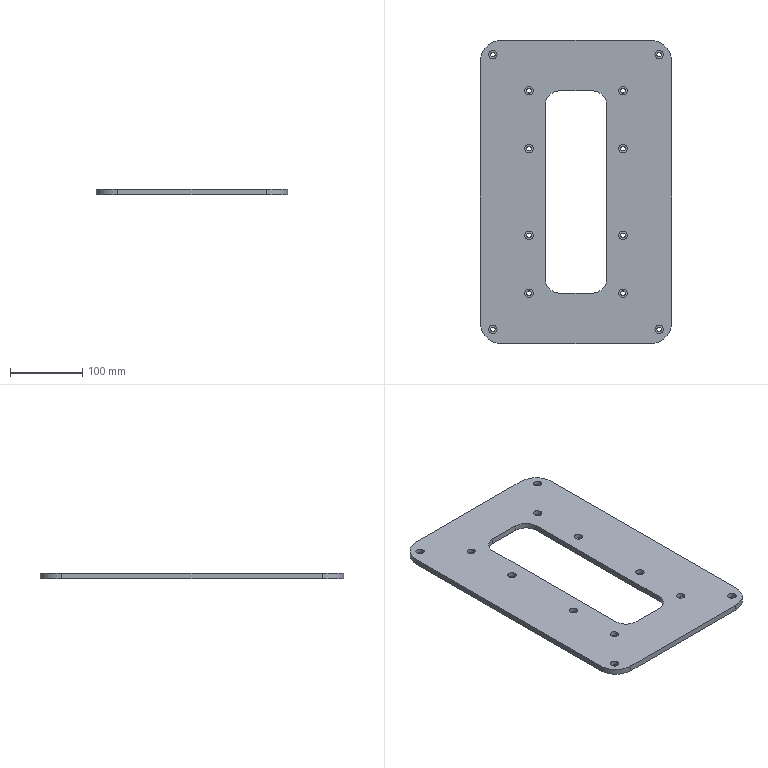Part | STEP file | SL2-MOLD_id354_xmt_txt | 1 solid | 54 faces | box 265 x 420 x 8 mm | volume 688291 mm3 | cylinder 32 | plane 22 | commonest cylinder face diameters 6.5 x12 11.5 x12 40 x4 60 x4
STEP:
#1=CARTESIAN_POINT('',(-42.5,-30.,101.));
#2=VERTEX_POINT('',#1);
#3=CARTESIAN_POINT('',(-42.5,210.,101.));
#4=VERTEX_POINT('',#3);
#5=CARTESIAN_POINT('',(-42.5,-30.,101.));
#6=DIRECTION('',(0.,1.,0.));
#7=VECTOR('',#6,1.);
#8=LINE('',#5,#7);
#9=EDGE_CURVE('',#2,#4,#8,.T.);
#10=ORIENTED_EDGE('',*,*,#9,.F.);
#11=CARTESIAN_POINT('',(-42.5,-30.,93.));
#12=VERTEX_POINT('',#11);
#13=CARTESIAN_POINT('',(-42.5,-30.,93.));
#14=DIRECTION('',(0.,0.,1.));
#15=VECTOR('',#14,1.);
#16=LINE('',#13,#15);
#17=EDGE_CURVE('',#12,#2,#16,.T.);
#18=ORIENTED_EDGE('',*,*,#17,.F.);
#19=CARTESIAN_POINT('',(-42.5,210.,93.));
#20=VERTEX_POINT('',#19);
#21=CARTESIAN_POINT('',(-42.5,-30.,93.));
#22=DIRECTION('',(0.,1.,0.));
#23=VECTOR('',#22,1.);
#24=LINE('',#21,#23);
#25=EDGE_CURVE('',#12,#20,#24,.T.);
#26=ORIENTED_EDGE('',*,*,#25,.T.);
#27=CARTESIAN_POINT('',(-42.5,210.,93.));
#28=DIRECTION('',(0.,0.,1.));
#29=VECTOR('',#28,1.);
#30=LINE('',#27,#29);
#31=EDGE_CURVE('',#20,#4,#30,.T.);
#32=ORIENTED_EDGE('',*,*,#31,.T.);
#33=EDGE_LOOP('',(#10,#18,#26,#32));
#34=FACE_OUTER_BOUND('',#33,.T.);
#35=CARTESIAN_POINT('',(-42.5,-30.,93.));
#36=DIRECTION('',(1.,0.,0.));
#37=DIRECTION('',(0.,1.,0.));
#38=AXIS2_PLACEMENT_3D('',#35,#36,#37);
#39=PLANE('',#38);
#40=ADVANCED_FACE('',(#34),#39,.T.);
#41=CARTESIAN_POINT('',(-22.5,-50.,101.));
#42=VERTEX_POINT('',#41);
#43=CARTESIAN_POINT('',(-22.5,-30.,101.));
#44=DIRECTION('',(0.,0.,-1.));
#45=DIRECTION('',(1.,0.,0.));
#46=AXIS2_PLACEMENT_3D('',#43,#44,#45);
#47=CIRCLE('',#46,20.);
#48=EDGE_CURVE('',#42,#2,#47,.T.);
#49=ORIENTED_EDGE('',*,*,#48,.F.);
#50=CARTESIAN_POINT('',(-22.5,-50.,93.));
#51=VERTEX_POINT('',#50);
#52=CARTESIAN_POINT('',(-22.5,-50.,93.));
#53=DIRECTION('',(0.,0.,1.));
#54=VECTOR('',#53,1.);
#55=LINE('',#52,#54);
#56=EDGE_CURVE('',#51,#42,#55,.T.);
#57=ORIENTED_EDGE('',*,*,#56,.F.);
#58=CARTESIAN_POINT('',(-22.5,-30.,93.));
#59=DIRECTION('',(0.,0.,-1.));
#60=DIRECTION('',(1.,0.,0.));
#61=AXIS2_PLACEMENT_3D('',#58,#59,#60);
#62=CIRCLE('',#61,20.);
#63=EDGE_CURVE('',#51,#12,#62,.T.);
#64=ORIENTED_EDGE('',*,*,#63,.T.);
#65=ORIENTED_EDGE('',*,*,#17,.T.);
#66=EDGE_LOOP('',(#49,#57,#64,#65));
#67=FACE_OUTER_BOUND('',#66,.T.);
#68=CARTESIAN_POINT('',(-22.5,-30.,93.));
#69=DIRECTION('',(0.,0.,1.));
#70=DIRECTION('',(1.,0.,0.));
#71=AXIS2_PLACEMENT_3D('',#68,#69,#70);
#72=CYLINDRICAL_SURFACE('',#71,20.);
#73=ADVANCED_FACE('',(#67),#72,.F.);
#74=CARTESIAN_POINT('',(22.5,-50.,101.));
#75=VERTEX_POINT('',#74);
#76=CARTESIAN_POINT('',(22.5,-50.,101.));
#77=DIRECTION('',(-1.,0.,0.));
#78=VECTOR('',#77,1.);
#79=LINE('',#76,#78);
#80=EDGE_CURVE('',#75,#42,#79,.T.);
#81=ORIENTED_EDGE('',*,*,#80,.F.);
#82=CARTESIAN_POINT('',(22.5,-50.,93.));
#83=VERTEX_POINT('',#82);
#84=CARTESIAN_POINT('',(22.5,-50.,93.));
#85=DIRECTION('',(0.,0.,1.));
#86=VECTOR('',#85,1.);
#87=LINE('',#84,#86);
#88=EDGE_CURVE('',#83,#75,#87,.T.);
#89=ORIENTED_EDGE('',*,*,#88,.F.);
#90=CARTESIAN_POINT('',(22.5,-50.,93.));
#91=DIRECTION('',(-1.,0.,0.));
#92=VECTOR('',#91,1.);
#93=LINE('',#90,#92);
#94=EDGE_CURVE('',#83,#51,#93,.T.);
#95=ORIENTED_EDGE('',*,*,#94,.T.);
#96=ORIENTED_EDGE('',*,*,#56,.T.);
#97=EDGE_LOOP('',(#81,#89,#95,#96));
#98=FACE_OUTER_BOUND('',#97,.T.);
#99=CARTESIAN_POINT('',(22.5,-50.,93.));
#100=DIRECTION('',(0.,1.,0.));
#101=DIRECTION('',(0.,0.,1.));
#102=AXIS2_PLACEMENT_3D('',#99,#100,#101);
#103=PLANE('',#102);
#104=ADVANCED_FACE('',(#98),#103,.T.);
#105=CARTESIAN_POINT('',(42.5,-30.,101.));
#106=VERTEX_POINT('',#105);
#107=CARTESIAN_POINT('',(22.5,-30.,101.));
#108=DIRECTION('',(0.,0.,-1.));
#109=DIRECTION('',(1.,0.,0.));
#110=AXIS2_PLACEMENT_3D('',#107,#108,#109);
#111=CIRCLE('',#110,20.);
#112=EDGE_CURVE('',#106,#75,#111,.T.);
#113=ORIENTED_EDGE('',*,*,#112,.F.);
#114=CARTESIAN_POINT('',(42.5,-30.,93.));
#115=VERTEX_POINT('',#114);
#116=CARTESIAN_POINT('',(42.5,-30.,93.));
#117=DIRECTION('',(0.,0.,1.));
#118=VECTOR('',#117,1.);
#119=LINE('',#116,#118);
#120=EDGE_CURVE('',#115,#106,#119,.T.);
#121=ORIENTED_EDGE('',*,*,#120,.F.);
#122=CARTESIAN_POINT('',(22.5,-30.,93.));
#123=DIRECTION('',(0.,0.,-1.));
#124=DIRECTION('',(1.,0.,0.));
#125=AXIS2_PLACEMENT_3D('',#122,#123,#124);
#126=CIRCLE('',#125,20.);
#127=EDGE_CURVE('',#115,#83,#126,.T.);
#128=ORIENTED_EDGE('',*,*,#127,.T.);
#129=ORIENTED_EDGE('',*,*,#88,.T.);
#130=EDGE_LOOP('',(#113,#121,#128,#129));
#131=FACE_OUTER_BOUND('',#130,.T.);
#132=CARTESIAN_POINT('',(22.5,-30.,93.));
#133=DIRECTION('',(0.,0.,1.));
#134=DIRECTION('',(1.,0.,0.));
#135=AXIS2_PLACEMENT_3D('',#132,#133,#134);
#136=CYLINDRICAL_SURFACE('',#135,20.);
#137=ADVANCED_FACE('',(#131),#136,.F.);
#138=CARTESIAN_POINT('',(42.5,210.,101.));
#139=VERTEX_POINT('',#138);
#140=CARTESIAN_POINT('',(42.5,210.,101.));
#141=DIRECTION('',(0.,-1.,0.));
#142=VECTOR('',#141,1.);
#143=LINE('',#140,#142);
#144=EDGE_CURVE('',#139,#106,#143,.T.);
#145=ORIENTED_EDGE('',*,*,#144,.F.);
#146=CARTESIAN_POINT('',(42.5,210.,93.));
#147=VERTEX_POINT('',#146);
#148=CARTESIAN_POINT('',(42.5,210.,93.));
#149=DIRECTION('',(0.,0.,1.));
#150=VECTOR('',#149,1.);
#151=LINE('',#148,#150);
#152=EDGE_CURVE('',#147,#139,#151,.T.);
#153=ORIENTED_EDGE('',*,*,#152,.F.);
#154=CARTESIAN_POINT('',(42.5,210.,93.));
#155=DIRECTION('',(0.,-1.,0.));
#156=VECTOR('',#155,1.);
#157=LINE('',#154,#156);
#158=EDGE_CURVE('',#147,#115,#157,.T.);
#159=ORIENTED_EDGE('',*,*,#158,.T.);
#160=ORIENTED_EDGE('',*,*,#120,.T.);
#161=EDGE_LOOP('',(#145,#153,#159,#160));
#162=FACE_OUTER_BOUND('',#161,.T.);
#163=CARTESIAN_POINT('',(42.5,210.,93.));
#164=DIRECTION('',(-1.,0.,0.));
#165=DIRECTION('',(0.,-1.,0.));
#166=AXIS2_PLACEMENT_3D('',#163,#164,#165);
#167=PLANE('',#166);
#168=ADVANCED_FACE('',(#162),#167,.T.);
#169=CARTESIAN_POINT('',(22.5,230.,101.));
#170=VERTEX_POINT('',#169);
#171=CARTESIAN_POINT('',(22.5,210.,101.));
#172=DIRECTION('',(0.,0.,-1.));
#173=DIRECTION('',(1.,0.,0.));
#174=AXIS2_PLACEMENT_3D('',#171,#172,#173);
#175=CIRCLE('',#174,20.);
#176=EDGE_CURVE('',#170,#139,#175,.T.);
#177=ORIENTED_EDGE('',*,*,#176,.F.);
#178=CARTESIAN_POINT('',(22.5,230.,93.));
#179=VERTEX_POINT('',#178);
#180=CARTESIAN_POINT('',(22.5,230.,93.));
#181=DIRECTION('',(0.,0.,1.));
#182=VECTOR('',#181,1.);
#183=LINE('',#180,#182);
#184=EDGE_CURVE('',#179,#170,#183,.T.);
#185=ORIENTED_EDGE('',*,*,#184,.F.);
#186=CARTESIAN_POINT('',(22.5,210.,93.));
#187=DIRECTION('',(0.,0.,-1.));
#188=DIRECTION('',(1.,0.,0.));
#189=AXIS2_PLACEMENT_3D('',#186,#187,#188);
#190=CIRCLE('',#189,20.);
#191=EDGE_CURVE('',#179,#147,#190,.T.);
#192=ORIENTED_EDGE('',*,*,#191,.T.);
#193=ORIENTED_EDGE('',*,*,#152,.T.);
#194=EDGE_LOOP('',(#177,#185,#192,#193));
#195=FACE_OUTER_BOUND('',#194,.T.);
#196=CARTESIAN_POINT('',(22.5,210.,93.));
#197=DIRECTION('',(0.,0.,1.));
#198=DIRECTION('',(1.,0.,0.));
#199=AXIS2_PLACEMENT_3D('',#196,#197,#198);
#200=CYLINDRICAL_SURFACE('',#199,20.);
#201=ADVANCED_FACE('',(#195),#200,.F.);
#202=CARTESIAN_POINT('',(-22.5,230.,101.));
#203=VERTEX_POINT('',#202);
#204=CARTESIAN_POINT('',(-22.5,230.,101.));
#205=DIRECTION('',(1.,0.,0.));
#206=VECTOR('',#205,1.);
#207=LINE('',#204,#206);
#208=EDGE_CURVE('',#203,#170,#207,.T.);
#209=ORIENTED_EDGE('',*,*,#208,.F.);
#210=CARTESIAN_POINT('',(-22.5,230.,93.));
#211=VERTEX_POINT('',#210);
#212=CARTESIAN_POINT('',(-22.5,230.,93.));
#213=DIRECTION('',(0.,0.,1.));
#214=VECTOR('',#213,1.);
#215=LINE('',#212,#214);
#216=EDGE_CURVE('',#211,#203,#215,.T.);
#217=ORIENTED_EDGE('',*,*,#216,.F.);
#218=CARTESIAN_POINT('',(-22.5,230.,93.));
#219=DIRECTION('',(1.,0.,0.));
#220=VECTOR('',#219,1.);
#221=LINE('',#218,#220);
#222=EDGE_CURVE('',#211,#179,#221,.T.);
#223=ORIENTED_EDGE('',*,*,#222,.T.);
#224=ORIENTED_EDGE('',*,*,#184,.T.);
#225=EDGE_LOOP('',(#209,#217,#223,#224));
#226=FACE_OUTER_BOUND('',#225,.T.);
#227=CARTESIAN_POINT('',(-22.5,230.,93.));
#228=DIRECTION('',(0.,-1.,0.));
#229=DIRECTION('',(0.,0.,-1.));
#230=AXIS2_PLACEMENT_3D('',#227,#228,#229);
#231=PLANE('',#230);
#232=ADVANCED_FACE('',(#226),#231,.T.);
#233=CARTESIAN_POINT('',(-102.5,300.,101.));
#234=VERTEX_POINT('',#233);
#235=CARTESIAN_POINT('',(102.5,300.,101.));
#236=VERTEX_POINT('',#235);
#237=CARTESIAN_POINT('',(-102.5,300.,101.));
#238=DIRECTION('',(1.,0.,0.));
#239=VECTOR('',#238,1.);
#240=LINE('',#237,#239);
#241=EDGE_CURVE('',#234,#236,#240,.T.);
#242=ORIENTED_EDGE('',*,*,#241,.T.);
#243=CARTESIAN_POINT('',(102.5,300.,93.));
#244=VERTEX_POINT('',#243);
#245=CARTESIAN_POINT('',(102.5,300.,93.));
#246=DIRECTION('',(0.,0.,1.));
#247=VECTOR('',#246,1.);
#248=LINE('',#245,#247);
#249=EDGE_CURVE('',#244,#236,#248,.T.);
#250=ORIENTED_EDGE('',*,*,#249,.F.);
#251=CARTESIAN_POINT('',(-102.5,300.,93.));
#252=VERTEX_POINT('',#251);
#253=CARTESIAN_POINT('',(-102.5,300.,93.));
#254=DIRECTION('',(1.,0.,0.));
#255=VECTOR('',#254,1.);
#256=LINE('',#253,#255);
#257=EDGE_CURVE('',#252,#244,#256,.T.);
#258=ORIENTED_EDGE('',*,*,#257,.F.);
#259=CARTESIAN_POINT('',(-102.5,300.,93.));
#260=DIRECTION('',(0.,0.,1.));
#261=VECTOR('',#260,1.);
#262=LINE('',#259,#261);
#263=EDGE_CURVE('',#252,#234,#262,.T.);
#264=ORIENTED_EDGE('',*,*,#263,.T.);
#265=EDGE_LOOP('',(#242,#250,#258,#264));
#266=FACE_OUTER_BOUND('',#265,.T.);
#267=CARTESIAN_POINT('',(-102.5,300.,93.));
#268=DIRECTION('',(0.,-1.,0.));
#269=DIRECTION('',(0.,0.,-1.));
#270=AXIS2_PLACEMENT_3D('',#267,#268,#269);
#271=PLANE('',#270);
#272=ADVANCED_FACE('',(#266),#271,.F.);
#273=CARTESIAN_POINT('',(132.5,270.,101.));
#274=VERTEX_POINT('',#273);
#275=CARTESIAN_POINT('',(102.5,270.,101.));
#276=DIRECTION('',(0.,0.,-1.));
#277=DIRECTION('',(1.,0.,0.));
#278=AXIS2_PLACEMENT_3D('',#275,#276,#277);
#279=CIRCLE('',#278,30.);
#280=EDGE_CURVE('',#236,#274,#279,.T.);
#281=ORIENTED_EDGE('',*,*,#280,.T.);
#282=CARTESIAN_POINT('',(132.5,270.,93.));
#283=VERTEX_POINT('',#282);
#284=CARTESIAN_POINT('',(132.5,270.,93.));
#285=DIRECTION('',(0.,0.,1.));
#286=VECTOR('',#285,1.);
#287=LINE('',#284,#286);
#288=EDGE_CURVE('',#283,#274,#287,.T.);
#289=ORIENTED_EDGE('',*,*,#288,.F.);
#290=CARTESIAN_POINT('',(102.5,270.,93.));
#291=DIRECTION('',(0.,0.,-1.));
#292=DIRECTION('',(1.,0.,0.));
#293=AXIS2_PLACEMENT_3D('',#290,#291,#292);
#294=CIRCLE('',#293,30.);
#295=EDGE_CURVE('',#244,#283,#294,.T.);
#296=ORIENTED_EDGE('',*,*,#295,.F.);
#297=ORIENTED_EDGE('',*,*,#249,.T.);
#298=EDGE_LOOP('',(#281,#289,#296,#297));
#299=FACE_OUTER_BOUND('',#298,.T.);
#300=CARTESIAN_POINT('',(102.5,270.,93.));
#301=DIRECTION('',(0.,0.,1.));
#302=DIRECTION('',(1.,0.,0.));
#303=AXIS2_PLACEMENT_3D('',#300,#301,#302);
#304=CYLINDRICAL_SURFACE('',#303,30.);
#305=ADVANCED_FACE('',(#299),#304,.T.);
#306=CARTESIAN_POINT('',(132.5,-90.,101.));
#307=VERTEX_POINT('',#306);
#308=CARTESIAN_POINT('',(132.5,270.,101.));
#309=DIRECTION('',(0.,-1.,0.));
#310=VECTOR('',#309,1.);
#311=LINE('',#308,#310);
#312=EDGE_CURVE('',#274,#307,#311,.T.);
#313=ORIENTED_EDGE('',*,*,#312,.T.);
#314=CARTESIAN_POINT('',(132.5,-90.,93.));
#315=VERTEX_POINT('',#314);
#316=CARTESIAN_POINT('',(132.5,-90.,93.));
#317=DIRECTION('',(0.,0.,1.));
#318=VECTOR('',#317,1.);
#319=LINE('',#316,#318);
#320=EDGE_CURVE('',#315,#307,#319,.T.);
#321=ORIENTED_EDGE('',*,*,#320,.F.);
#322=CARTESIAN_POINT('',(132.5,270.,93.));
#323=DIRECTION('',(0.,-1.,0.));
#324=VECTOR('',#323,1.);
#325=LINE('',#322,#324);
#326=EDGE_CURVE('',#283,#315,#325,.T.);
#327=ORIENTED_EDGE('',*,*,#326,.F.);
#328=ORIENTED_EDGE('',*,*,#288,.T.);
#329=EDGE_LOOP('',(#313,#321,#327,#328));
#330=FACE_OUTER_BOUND('',#329,.T.);
#331=CARTESIAN_POINT('',(132.5,270.,93.));
#332=DIRECTION('',(-1.,0.,0.));
#333=DIRECTION('',(0.,-1.,0.));
#334=AXIS2_PLACEMENT_3D('',#331,#332,#333);
#335=PLANE('',#334);
#336=ADVANCED_FACE('',(#330),#335,.F.);
#337=CARTESIAN_POINT('',(102.5,-120.,101.));
#338=VERTEX_POINT('',#337);
#339=CARTESIAN_POINT('',(102.5,-90.,101.));
#340=DIRECTION('',(0.,0.,-1.));
#341=DIRECTION('',(1.,0.,0.));
#342=AXIS2_PLACEMENT_3D('',#339,#340,#341);
#343=CIRCLE('',#342,30.);
#344=EDGE_CURVE('',#307,#338,#343,.T.);
#345=ORIENTED_EDGE('',*,*,#344,.T.);
#346=CARTESIAN_POINT('',(102.5,-120.,93.));
#347=VERTEX_POINT('',#346);
#348=CARTESIAN_POINT('',(102.5,-120.,93.));
#349=DIRECTION('',(0.,0.,1.));
#350=VECTOR('',#349,1.);
#351=LINE('',#348,#350);
#352=EDGE_CURVE('',#347,#338,#351,.T.);
#353=ORIENTED_EDGE('',*,*,#352,.F.);
#354=CARTESIAN_POINT('',(102.5,-90.,93.));
#355=DIRECTION('',(0.,0.,-1.));
#356=DIRECTION('',(1.,0.,0.));
#357=AXIS2_PLACEMENT_3D('',#354,#355,#356);
#358=CIRCLE('',#357,30.);
#359=EDGE_CURVE('',#315,#347,#358,.T.);
#360=ORIENTED_EDGE('',*,*,#359,.F.);
#361=ORIENTED_EDGE('',*,*,#320,.T.);
#362=EDGE_LOOP('',(#345,#353,#360,#361));
#363=FACE_OUTER_BOUND('',#362,.T.);
#364=CARTESIAN_POINT('',(102.5,-90.,93.));
#365=DIRECTION('',(0.,0.,1.));
#366=DIRECTION('',(1.,0.,0.));
#367=AXIS2_PLACEMENT_3D('',#364,#365,#366);
#368=CYLINDRICAL_SURFACE('',#367,30.);
#369=ADVANCED_FACE('',(#363),#368,.T.);
#370=CARTESIAN_POINT('',(-102.5,-120.,101.));
#371=VERTEX_POINT('',#370);
#372=CARTESIAN_POINT('',(102.5,-120.,101.));
#373=DIRECTION('',(-1.,0.,0.));
#374=VECTOR('',#373,1.);
#375=LINE('',#372,#374);
#376=EDGE_CURVE('',#338,#371,#375,.T.);
#377=ORIENTED_EDGE('',*,*,#376,.T.);
#378=CARTESIAN_POINT('',(-102.5,-120.,93.));
#379=VERTEX_POINT('',#378);
#380=CARTESIAN_POINT('',(-102.5,-120.,93.));
#381=DIRECTION('',(0.,0.,1.));
#382=VECTOR('',#381,1.);
#383=LINE('',#380,#382);
#384=EDGE_CURVE('',#379,#371,#383,.T.);
#385=ORIENTED_EDGE('',*,*,#384,.F.);
#386=CARTESIAN_POINT('',(102.5,-120.,93.));
#387=DIRECTION('',(-1.,0.,0.));
#388=VECTOR('',#387,1.);
#389=LINE('',#386,#388);
#390=EDGE_CURVE('',#347,#379,#389,.T.);
#391=ORIENTED_EDGE('',*,*,#390,.F.);
#392=ORIENTED_EDGE('',*,*,#352,.T.);
#393=EDGE_LOOP('',(#377,#385,#391,#392));
#394=FACE_OUTER_BOUND('',#393,.T.);
#395=CARTESIAN_POINT('',(102.5,-120.,93.));
#396=DIRECTION('',(0.,1.,0.));
#397=DIRECTION('',(0.,0.,1.));
#398=AXIS2_PLACEMENT_3D('',#395,#396,#397);
#399=PLANE('',#398);
#400=ADVANCED_FACE('',(#394),#399,.F.);
#401=CARTESIAN_POINT('',(-132.5,-90.,101.));
#402=VERTEX_POINT('',#401);
#403=CARTESIAN_POINT('',(-102.5,-90.,101.));
#404=DIRECTION('',(0.,0.,-1.));
#405=DIRECTION('',(1.,0.,0.));
#406=AXIS2_PLACEMENT_3D('',#403,#404,#405);
#407=CIRCLE('',#406,30.);
#408=EDGE_CURVE('',#371,#402,#407,.T.);
#409=ORIENTED_EDGE('',*,*,#408,.T.);
#410=CARTESIAN_POINT('',(-132.5,-90.,93.));
#411=VERTEX_POINT('',#410);
#412=CARTESIAN_POINT('',(-132.5,-90.,93.));
#413=DIRECTION('',(0.,0.,1.));
#414=VECTOR('',#413,1.);
#415=LINE('',#412,#414);
#416=EDGE_CURVE('',#411,#402,#415,.T.);
#417=ORIENTED_EDGE('',*,*,#416,.F.);
#418=CARTESIAN_POINT('',(-102.5,-90.,93.));
#419=DIRECTION('',(0.,0.,-1.));
#420=DIRECTION('',(1.,0.,0.));
#421=AXIS2_PLACEMENT_3D('',#418,#419,#420);
#422=CIRCLE('',#421,30.);
#423=EDGE_CURVE('',#379,#411,#422,.T.);
#424=ORIENTED_EDGE('',*,*,#423,.F.);
#425=ORIENTED_EDGE('',*,*,#384,.T.);
#426=EDGE_LOOP('',(#409,#417,#424,#425));
#427=FACE_OUTER_BOUND('',#426,.T.);
#428=CARTESIAN_POINT('',(-102.5,-90.,93.));
#429=DIRECTION('',(0.,0.,1.));
#430=DIRECTION('',(1.,0.,0.));
#431=AXIS2_PLACEMENT_3D('',#428,#429,#430);
#432=CYLINDRICAL_SURFACE('',#431,30.);
#433=ADVANCED_FACE('',(#427),#432,.T.);
#434=CARTESIAN_POINT('',(-132.5,270.,101.));
#435=VERTEX_POINT('',#434);
#436=CARTESIAN_POINT('',(-132.5,-90.,101.));
#437=DIRECTION('',(0.,1.,0.));
#438=VECTOR('',#437,1.);
#439=LINE('',#436,#438);
#440=EDGE_CURVE('',#402,#435,#439,.T.);
#441=ORIENTED_EDGE('',*,*,#440,.T.);
#442=CARTESIAN_POINT('',(-132.5,270.,93.));
#443=VERTEX_POINT('',#442);
#444=CARTESIAN_POINT('',(-132.5,270.,93.));
#445=DIRECTION('',(0.,0.,1.));
#446=VECTOR('',#445,1.);
#447=LINE('',#444,#446);
#448=EDGE_CURVE('',#443,#435,#447,.T.);
#449=ORIENTED_EDGE('',*,*,#448,.F.);
#450=CARTESIAN_POINT('',(-132.5,-90.,93.));
#451=DIRECTION('',(0.,1.,0.));
#452=VECTOR('',#451,1.);
#453=LINE('',#450,#452);
#454=EDGE_CURVE('',#411,#443,#453,.T.);
#455=ORIENTED_EDGE('',*,*,#454,.F.);
#456=ORIENTED_EDGE('',*,*,#416,.T.);
#457=EDGE_LOOP('',(#441,#449,#455,#456));
#458=FACE_OUTER_BOUND('',#457,.T.);
#459=CARTESIAN_POINT('',(-132.5,-90.,93.));
#460=DIRECTION('',(1.,0.,0.));
#461=DIRECTION('',(0.,1.,0.));
#462=AXIS2_PLACEMENT_3D('',#459,#460,#461);
#463=PLANE('',#462);
#464=ADVANCED_FACE('',(#458),#463,.F.);
#465=CARTESIAN_POINT('',(-102.5,270.,101.));
#466=DIRECTION('',(0.,0.,-1.));
#467=DIRECTION('',(1.,0.,0.));
#468=AXIS2_PLACEMENT_3D('',#465,#466,#467);
#469=CIRCLE('',#468,30.);
#470=EDGE_CURVE('',#435,#234,#469,.T.);
#471=ORIENTED_EDGE('',*,*,#470,.T.);
#472=ORIENTED_EDGE('',*,*,#263,.F.);
#473=CARTESIAN_POINT('',(-102.5,270.,93.));
#474=DIRECTION('',(0.,0.,-1.));
#475=DIRECTION('',(1.,0.,0.));
#476=AXIS2_PLACEMENT_3D('',#473,#474,#475);
#477=CIRCLE('',#476,30.);
#478=EDGE_CURVE('',#443,#252,#477,.T.);
#479=ORIENTED_EDGE('',*,*,#478,.F.);
#480=ORIENTED_EDGE('',*,*,#448,.T.);
#481=EDGE_LOOP('',(#471,#472,#479,#480));
#482=FACE_OUTER_BOUND('',#481,.T.);
#483=CARTESIAN_POINT('',(-102.5,270.,93.));
#484=DIRECTION('',(0.,0.,1.));
#485=DIRECTION('',(1.,0.,0.));
#486=AXIS2_PLACEMENT_3D('',#483,#484,#485);
#487=CYLINDRICAL_SURFACE('',#486,30.);
#488=ADVANCED_FACE('',(#482),#487,.T.);
#489=CARTESIAN_POINT('',(-22.5,210.,101.));
#490=DIRECTION('',(0.,0.,-1.));
#491=DIRECTION('',(1.,0.,0.));
#492=AXIS2_PLACEMENT_3D('',#489,#490,#491);
#493=CIRCLE('',#492,20.);
#494=EDGE_CURVE('',#4,#203,#493,.T.);
#495=ORIENTED_EDGE('',*,*,#494,.F.);
#496=ORIENTED_EDGE('',*,*,#31,.F.);
#497=CARTESIAN_POINT('',(-22.5,210.,93.));
#498=DIRECTION('',(0.,0.,-1.));
#499=DIRECTION('',(1.,0.,0.));
#500=AXIS2_PLACEMENT_3D('',#497,#498,#499);
#501=CIRCLE('',#500,20.);
#502=EDGE_CURVE('',#20,#211,#501,.T.);
#503=ORIENTED_EDGE('',*,*,#502,.T.);
#504=ORIENTED_EDGE('',*,*,#216,.T.);
#505=EDGE_LOOP('',(#495,#496,#503,#504));
#506=FACE_OUTER_BOUND('',#505,.T.);
#507=CARTESIAN_POINT('',(-22.5,210.,93.));
#508=DIRECTION('',(0.,0.,1.));
#509=DIRECTION('',(1.,0.,0.));
#510=AXIS2_PLACEMENT_3D('',#507,#508,#509);
#511=CYLINDRICAL_SURFACE('',#510,20.);
#512=ADVANCED_FACE('',(#506),#511,.F.);
#513=CARTESIAN_POINT('',(-118.25,280.,93.));
#514=VERTEX_POINT('',#513);
#515=CARTESIAN_POINT('',(-115.,280.,93.));
#516=DIRECTION('',(0.,0.,-1.));
#517=DIRECTION('',(-1.,0.,0.));
#518=AXIS2_PLACEMENT_3D('',#515,#516,#517);
#519=CIRCLE('',#518,3.25);
#520=EDGE_CURVE('',#514,#514,#519,.T.);
#521=ORIENTED_EDGE('',*,*,#520,.F.);
#522=EDGE_LOOP('',(#521));
#523=FACE_BOUND('',#522,.T.);
#524=CARTESIAN_POINT('',(111.75,-100.,93.));
#525=VERTEX_POINT('',#524);
#526=CARTESIAN_POINT('',(115.,-100.,93.));
#527=DIRECTION('',(0.,0.,-1.));
#528=DIRECTION('',(-1.,0.,0.));
#529=AXIS2_PLACEMENT_3D('',#526,#527,#528);
#530=CIRCLE('',#529,3.25);
#531=EDGE_CURVE('',#525,#525,#530,.T.);
#532=ORIENTED_EDGE('',*,*,#531,.F.);
#533=EDGE_LOOP('',(#532));
#534=FACE_BOUND('',#533,.T.);
#535=CARTESIAN_POINT('',(-68.25,230.,93.));
#536=VERTEX_POINT('',#535);
#537=CARTESIAN_POINT('',(-65.,230.,93.));
#538=DIRECTION('',(0.,0.,-1.));
#539=DIRECTION('',(-1.,0.,0.));
#540=AXIS2_PLACEMENT_3D('',#537,#538,#539);
#541=CIRCLE('',#540,3.25);
#542=EDGE_CURVE('',#536,#536,#541,.T.);
#543=ORIENTED_EDGE('',*,*,#542,.F.);
#544=EDGE_LOOP('',(#543));
#545=FACE_BOUND('',#544,.T.);
#546=CARTESIAN_POINT('',(-68.25,150.,93.));
#547=VERTEX_POINT('',#546);
#548=CARTESIAN_POINT('',(-65.,150.,93.));
#549=DIRECTION('',(0.,0.,-1.));
#550=DIRECTION('',(-1.,0.,0.));
#551=AXIS2_PLACEMENT_3D('',#548,#549,#550);
#552=CIRCLE('',#551,3.25);
#553=EDGE_CURVE('',#547,#547,#552,.T.);
#554=ORIENTED_EDGE('',*,*,#553,.F.);
#555=EDGE_LOOP('',(#554));
#556=FACE_BOUND('',#555,.T.);
#557=CARTESIAN_POINT('',(-68.25,30.,93.));
#558=VERTEX_POINT('',#557);
#559=CARTESIAN_POINT('',(-65.,30.,93.));
#560=DIRECTION('',(0.,0.,-1.));
#561=DIRECTION('',(-1.,0.,0.));
#562=AXIS2_PLACEMENT_3D('',#559,#560,#561);
#563=CIRCLE('',#562,3.25);
#564=EDGE_CURVE('',#558,#558,#563,.T.);
#565=ORIENTED_EDGE('',*,*,#564,.F.);
#566=EDGE_LOOP('',(#565));
#567=FACE_BOUND('',#566,.T.);
#568=CARTESIAN_POINT('',(-118.25,-100.,93.));
#569=VERTEX_POINT('',#568);
#570=CARTESIAN_POINT('',(-115.,-100.,93.));
#571=DIRECTION('',(0.,0.,-1.));
#572=DIRECTION('',(-1.,0.,0.));
#573=AXIS2_PLACEMENT_3D('',#570,#571,#572);
#574=CIRCLE('',#573,3.25);
#575=EDGE_CURVE('',#569,#569,#574,.T.);
#576=ORIENTED_EDGE('',*,*,#575,.F.);
#577=EDGE_LOOP('',(#576));
#578=FACE_BOUND('',#577,.T.);
#579=CARTESIAN_POINT('',(-68.25,-50.,93.));
#580=VERTEX_POINT('',#579);
#581=CARTESIAN_POINT('',(-65.,-50.,93.));
#582=DIRECTION('',(0.,0.,-1.));
#583=DIRECTION('',(-1.,0.,0.));
#584=AXIS2_PLACEMENT_3D('',#581,#582,#583);
#585=CIRCLE('',#584,3.25);
#586=EDGE_CURVE('',#580,#580,#585,.T.);
#587=ORIENTED_EDGE('',*,*,#586,.F.);
#588=EDGE_LOOP('',(#587));
#589=FACE_BOUND('',#588,.T.);
#590=CARTESIAN_POINT('',(61.75,-50.,93.));
#591=VERTEX_POINT('',#590);
#592=CARTESIAN_POINT('',(65.,-50.,93.));
#593=DIRECTION('',(0.,0.,-1.));
#594=DIRECTION('',(-1.,0.,0.));
#595=AXIS2_PLACEMENT_3D('',#592,#593,#594);
#596=CIRCLE('',#595,3.25);
#597=EDGE_CURVE('',#591,#591,#596,.T.);
#598=ORIENTED_EDGE('',*,*,#597,.F.);
#599=EDGE_LOOP('',(#598));
#600=FACE_BOUND('',#599,.T.);
#601=CARTESIAN_POINT('',(61.75,30.,93.));
#602=VERTEX_POINT('',#601);
#603=CARTESIAN_POINT('',(65.,30.,93.));
#604=DIRECTION('',(0.,0.,-1.));
#605=DIRECTION('',(-1.,0.,0.));
#606=AXIS2_PLACEMENT_3D('',#603,#604,#605);
#607=CIRCLE('',#606,3.25);
#608=EDGE_CURVE('',#602,#602,#607,.T.);
#609=ORIENTED_EDGE('',*,*,#608,.F.);
#610=EDGE_LOOP('',(#609));
#611=FACE_BOUND('',#610,.T.);
#612=CARTESIAN_POINT('',(61.75,150.,93.));
#613=VERTEX_POINT('',#612);
#614=CARTESIAN_POINT('',(65.,150.,93.));
#615=DIRECTION('',(0.,0.,-1.));
#616=DIRECTION('',(-1.,0.,0.));
#617=AXIS2_PLACEMENT_3D('',#614,#615,#616);
#618=CIRCLE('',#617,3.25);
#619=EDGE_CURVE('',#613,#613,#618,.T.);
#620=ORIENTED_EDGE('',*,*,#619,.F.);
#621=EDGE_LOOP('',(#620));
#622=FACE_BOUND('',#621,.T.);
#623=CARTESIAN_POINT('',(61.75,230.,93.));
#624=VERTEX_POINT('',#623);
#625=CARTESIAN_POINT('',(65.,230.,93.));
#626=DIRECTION('',(0.,0.,-1.));
#627=DIRECTION('',(-1.,0.,0.));
#628=AXIS2_PLACEMENT_3D('',#625,#626,#627);
#629=CIRCLE('',#628,3.25);
#630=EDGE_CURVE('',#624,#624,#629,.T.);
#631=ORIENTED_EDGE('',*,*,#630,.F.);
#632=EDGE_LOOP('',(#631));
#633=FACE_BOUND('',#632,.T.);
#634=CARTESIAN_POINT('',(111.75,280.,93.));
#635=VERTEX_POINT('',#634);
#636=CARTESIAN_POINT('',(115.,280.,93.));
#637=DIRECTION('',(0.,0.,-1.));
#638=DIRECTION('',(-1.,0.,0.));
#639=AXIS2_PLACEMENT_3D('',#636,#637,#638);
#640=CIRCLE('',#639,3.25);
#641=EDGE_CURVE('',#635,#635,#640,.T.);
#642=ORIENTED_EDGE('',*,*,#641,.F.);
#643=EDGE_LOOP('',(#642));
#644=FACE_BOUND('',#643,.T.);
#645=ORIENTED_EDGE('',*,*,#257,.T.);
#646=ORIENTED_EDGE('',*,*,#295,.T.);
#647=ORIENTED_EDGE('',*,*,#326,.T.);
#648=ORIENTED_EDGE('',*,*,#359,.T.);
#649=ORIENTED_EDGE('',*,*,#390,.T.);
#650=ORIENTED_EDGE('',*,*,#423,.T.);
#651=ORIENTED_EDGE('',*,*,#454,.T.);
#652=ORIENTED_EDGE('',*,*,#478,.T.);
#653=EDGE_LOOP('',(#645,#646,#647,#648,#649,#650,#651,#652));
#654=FACE_BOUND('',#653,.T.);
#655=ORIENTED_EDGE('',*,*,#25,.F.);
#656=ORIENTED_EDGE('',*,*,#63,.F.);
#657=ORIENTED_EDGE('',*,*,#94,.F.);
#658=ORIENTED_EDGE('',*,*,#127,.F.);
#659=ORIENTED_EDGE('',*,*,#158,.F.);
#660=ORIENTED_EDGE('',*,*,#191,.F.);
#661=ORIENTED_EDGE('',*,*,#222,.F.);
#662=ORIENTED_EDGE('',*,*,#502,.F.);
#663=EDGE_LOOP('',(#655,#656,#657,#658,#659,#660,#661,#662));
#664=FACE_BOUND('',#663,.T.);
#665=CARTESIAN_POINT('',(102.5,270.,93.));
#666=DIRECTION('',(0.,0.,-1.));
#667=DIRECTION('',(-1.,0.,0.));
#668=AXIS2_PLACEMENT_3D('',#665,#666,#667);
#669=PLANE('',#668);
#670=ADVANCED_FACE('',(#523,#534,#545,#556,#567,#578,#589,#600,#611,#622,#633,#644,#654,#664),#669,.T.);
#671=CARTESIAN_POINT('',(-120.75,280.,101.));
#672=VERTEX_POINT('',#671);
#673=CARTESIAN_POINT('',(-115.,280.,101.));
#674=DIRECTION('',(0.,0.,1.));
#675=DIRECTION('',(-1.,0.,0.));
#676=AXIS2_PLACEMENT_3D('',#673,#674,#675);
#677=CIRCLE('',#676,5.75);
#678=EDGE_CURVE('',#672,#672,#677,.T.);
#679=ORIENTED_EDGE('',*,*,#678,.F.);
#680=EDGE_LOOP('',(#679));
#681=FACE_BOUND('',#680,.T.);
#682=CARTESIAN_POINT('',(-70.75,230.,101.));
#683=VERTEX_POINT('',#682);
#684=CARTESIAN_POINT('',(-65.,230.,101.));
#685=DIRECTION('',(0.,0.,1.));
#686=DIRECTION('',(-1.,0.,0.));
#687=AXIS2_PLACEMENT_3D('',#684,#685,#686);
#688=CIRCLE('',#687,5.75);
#689=EDGE_CURVE('',#683,#683,#688,.T.);
#690=ORIENTED_EDGE('',*,*,#689,.F.);
#691=EDGE_LOOP('',(#690));
#692=FACE_BOUND('',#691,.T.);
#693=CARTESIAN_POINT('',(-70.75,150.,101.));
#694=VERTEX_POINT('',#693);
#695=CARTESIAN_POINT('',(-65.,150.,101.));
#696=DIRECTION('',(0.,0.,1.));
#697=DIRECTION('',(-1.,0.,0.));
#698=AXIS2_PLACEMENT_3D('',#695,#696,#697);
#699=CIRCLE('',#698,5.75);
#700=EDGE_CURVE('',#694,#694,#699,.T.);
#701=ORIENTED_EDGE('',*,*,#700,.F.);
#702=EDGE_LOOP('',(#701));
#703=FACE_BOUND('',#702,.T.);
#704=CARTESIAN_POINT('',(-70.75,30.,101.));
#705=VERTEX_POINT('',#704);
#706=CARTESIAN_POINT('',(-65.,30.,101.));
#707=DIRECTION('',(0.,0.,1.));
#708=DIRECTION('',(-1.,0.,0.));
#709=AXIS2_PLACEMENT_3D('',#706,#707,#708);
#710=CIRCLE('',#709,5.75);
#711=EDGE_CURVE('',#705,#705,#710,.T.);
#712=ORIENTED_EDGE('',*,*,#711,.F.);
#713=EDGE_LOOP('',(#712));
#714=FACE_BOUND('',#713,.T.);
#715=CARTESIAN_POINT('',(-70.75,-50.,101.));
#716=VERTEX_POINT('',#715);
#717=CARTESIAN_POINT('',(-65.,-50.,101.));
#718=DIRECTION('',(0.,0.,1.));
#719=DIRECTION('',(-1.,0.,0.));
#720=AXIS2_PLACEMENT_3D('',#717,#718,#719);
#721=CIRCLE('',#720,5.75);
#722=EDGE_CURVE('',#716,#716,#721,.T.);
#723=ORIENTED_EDGE('',*,*,#722,.F.);
#724=EDGE_LOOP('',(#723));
#725=FACE_BOUND('',#724,.T.);
#726=CARTESIAN_POINT('',(-120.75,-100.,101.));
#727=VERTEX_POINT('',#726);
#728=CARTESIAN_POINT('',(-115.,-100.,101.));
#729=DIRECTION('',(0.,0.,1.));
#730=DIRECTION('',(-1.,0.,0.));
#731=AXIS2_PLACEMENT_3D('',#728,#729,#730);
#732=CIRCLE('',#731,5.75);
#733=EDGE_CURVE('',#727,#727,#732,.T.);
#734=ORIENTED_EDGE('',*,*,#733,.F.);
#735=EDGE_LOOP('',(#734));
#736=FACE_BOUND('',#735,.T.);
#737=CARTESIAN_POINT('',(109.25,-100.,101.));
#738=VERTEX_POINT('',#737);
#739=CARTESIAN_POINT('',(115.,-100.,101.));
#740=DIRECTION('',(0.,0.,1.));
#741=DIRECTION('',(-1.,0.,0.));
#742=AXIS2_PLACEMENT_3D('',#739,#740,#741);
#743=CIRCLE('',#742,5.75);
#744=EDGE_CURVE('',#738,#738,#743,.T.);
#745=ORIENTED_EDGE('',*,*,#744,.F.);
#746=EDGE_LOOP('',(#745));
#747=FACE_BOUND('',#746,.T.);
#748=CARTESIAN_POINT('',(59.25,-50.,101.));
#749=VERTEX_POINT('',#748);
#750=CARTESIAN_POINT('',(65.,-50.,101.));
#751=DIRECTION('',(0.,0.,1.));
#752=DIRECTION('',(-1.,0.,0.));
#753=AXIS2_PLACEMENT_3D('',#750,#751,#752);
#754=CIRCLE('',#753,5.75);
#755=EDGE_CURVE('',#749,#749,#754,.T.);
#756=ORIENTED_EDGE('',*,*,#755,.F.);
#757=EDGE_LOOP('',(#756));
#758=FACE_BOUND('',#757,.T.);
#759=CARTESIAN_POINT('',(59.25,30.,101.));
#760=VERTEX_POINT('',#759);
#761=CARTESIAN_POINT('',(65.,30.,101.));
#762=DIRECTION('',(0.,0.,1.));
#763=DIRECTION('',(-1.,0.,0.));
#764=AXIS2_PLACEMENT_3D('',#761,#762,#763);
#765=CIRCLE('',#764,5.75);
#766=EDGE_CURVE('',#760,#760,#765,.T.);
#767=ORIENTED_EDGE('',*,*,#766,.F.);
#768=EDGE_LOOP('',(#767));
#769=FACE_BOUND('',#768,.T.);
#770=CARTESIAN_POINT('',(59.25,150.,101.));
#771=VERTEX_POINT('',#770);
#772=CARTESIAN_POINT('',(65.,150.,101.));
#773=DIRECTION('',(0.,0.,1.));
#774=DIRECTION('',(-1.,0.,0.));
#775=AXIS2_PLACEMENT_3D('',#772,#773,#774);
#776=CIRCLE('',#775,5.75);
#777=EDGE_CURVE('',#771,#771,#776,.T.);
#778=ORIENTED_EDGE('',*,*,#777,.F.);
#779=EDGE_LOOP('',(#778));
#780=FACE_BOUND('',#779,.T.);
#781=CARTESIAN_POINT('',(59.25,230.,101.));
#782=VERTEX_POINT('',#781);
#783=CARTESIAN_POINT('',(65.,230.,101.));
#784=DIRECTION('',(0.,0.,1.));
#785=DIRECTION('',(-1.,0.,0.));
#786=AXIS2_PLACEMENT_3D('',#783,#784,#785);
#787=CIRCLE('',#786,5.75);
#788=EDGE_CURVE('',#782,#782,#787,.T.);
#789=ORIENTED_EDGE('',*,*,#788,.F.);
#790=EDGE_LOOP('',(#789));
#791=FACE_BOUND('',#790,.T.);
#792=CARTESIAN_POINT('',(109.25,280.,101.));
#793=VERTEX_POINT('',#792);
#794=CARTESIAN_POINT('',(115.,280.,101.));
#795=DIRECTION('',(0.,0.,1.));
#796=DIRECTION('',(-1.,0.,0.));
#797=AXIS2_PLACEMENT_3D('',#794,#795,#796);
#798=CIRCLE('',#797,5.75);
#799=EDGE_CURVE('',#793,#793,#798,.T.);
#800=ORIENTED_EDGE('',*,*,#799,.F.);
#801=EDGE_LOOP('',(#800));
#802=FACE_BOUND('',#801,.T.);
#803=ORIENTED_EDGE('',*,*,#241,.F.);
#804=ORIENTED_EDGE('',*,*,#470,.F.);
#805=ORIENTED_EDGE('',*,*,#440,.F.);
#806=ORIENTED_EDGE('',*,*,#408,.F.);
#807=ORIENTED_EDGE('',*,*,#376,.F.);
#808=ORIENTED_EDGE('',*,*,#344,.F.);
#809=ORIENTED_EDGE('',*,*,#312,.F.);
#810=ORIENTED_EDGE('',*,*,#280,.F.);
#811=EDGE_LOOP('',(#803,#804,#805,#806,#807,#808,#809,#810));
#812=FACE_BOUND('',#811,.T.);
#813=ORIENTED_EDGE('',*,*,#9,.T.);
#814=ORIENTED_EDGE('',*,*,#494,.T.);
#815=ORIENTED_EDGE('',*,*,#208,.T.);
#816=ORIENTED_EDGE('',*,*,#176,.T.);
#817=ORIENTED_EDGE('',*,*,#144,.T.);
#818=ORIENTED_EDGE('',*,*,#112,.T.);
#819=ORIENTED_EDGE('',*,*,#80,.T.);
#820=ORIENTED_EDGE('',*,*,#48,.T.);
#821=EDGE_LOOP('',(#813,#814,#815,#816,#817,#818,#819,#820));
#822=FACE_BOUND('',#821,.T.);
#823=CARTESIAN_POINT('',(102.5,270.,101.));
#824=DIRECTION('',(0.,0.,-1.));
#825=DIRECTION('',(-1.,0.,0.));
#826=AXIS2_PLACEMENT_3D('',#823,#824,#825);
#827=PLANE('',#826);
#828=ADVANCED_FACE('',(#681,#692,#703,#714,#725,#736,#747,#758,#769,#780,#791,#802,#812,#822),#827,.F.);
#829=CARTESIAN_POINT('',(120.75,280.,95.));
#830=VERTEX_POINT('',#829);
#831=CARTESIAN_POINT('',(115.,280.,95.));
#832=DIRECTION('',(0.,0.,-1.));
#833=DIRECTION('',(1.,0.,0.));
#834=AXIS2_PLACEMENT_3D('',#831,#832,#833);
#835=CIRCLE('',#834,5.75);
#836=EDGE_CURVE('',#830,#830,#835,.T.);
#837=ORIENTED_EDGE('',*,*,#836,.T.);
#838=EDGE_LOOP('',(#837));
#839=FACE_BOUND('',#838,.T.);
#840=ORIENTED_EDGE('',*,*,#799,.T.);
#841=EDGE_LOOP('',(#840));
#842=FACE_BOUND('',#841,.T.);
#843=CARTESIAN_POINT('',(115.,280.,115.));
#844=DIRECTION('',(0.,0.,-1.));
#845=DIRECTION('',(-1.,0.,0.));
#846=AXIS2_PLACEMENT_3D('',#843,#844,#845);
#847=CYLINDRICAL_SURFACE('',#846,5.75);
#848=ADVANCED_FACE('',(#839,#842),#847,.F.);
#849=CARTESIAN_POINT('',(118.25,280.,95.));
#850=VERTEX_POINT('',#849);
#851=CARTESIAN_POINT('',(115.,280.,95.));
#852=DIRECTION('',(0.,0.,1.));
#853=DIRECTION('',(1.,0.,0.));
#854=AXIS2_PLACEMENT_3D('',#851,#852,#853);
#855=CIRCLE('',#854,3.25);
#856=EDGE_CURVE('',#850,#850,#855,.T.);
#857=ORIENTED_EDGE('',*,*,#856,.F.);
#858=EDGE_LOOP('',(#857));
#859=FACE_BOUND('',#858,.T.);
#860=ORIENTED_EDGE('',*,*,#836,.F.);
#861=EDGE_LOOP('',(#860));
#862=FACE_BOUND('',#861,.T.);
#863=CARTESIAN_POINT('',(115.,280.,95.));
#864=DIRECTION('',(0.,0.,1.));
#865=DIRECTION('',(1.,0.,0.));
#866=AXIS2_PLACEMENT_3D('',#863,#864,#865);
#867=PLANE('',#866);
#868=ADVANCED_FACE('',(#859,#862),#867,.T.);
#869=CARTESIAN_POINT('',(70.75,230.,95.));
#870=VERTEX_POINT('',#869);
#871=CARTESIAN_POINT('',(65.,230.,95.));
#872=DIRECTION('',(0.,0.,-1.));
#873=DIRECTION('',(1.,0.,0.));
#874=AXIS2_PLACEMENT_3D('',#871,#872,#873);
#875=CIRCLE('',#874,5.75);
#876=EDGE_CURVE('',#870,#870,#875,.T.);
#877=ORIENTED_EDGE('',*,*,#876,.T.);
#878=EDGE_LOOP('',(#877));
#879=FACE_BOUND('',#878,.T.);
#880=ORIENTED_EDGE('',*,*,#788,.T.);
#881=EDGE_LOOP('',(#880));
#882=FACE_BOUND('',#881,.T.);
#883=CARTESIAN_POINT('',(65.,230.,115.));
#884=DIRECTION('',(0.,0.,-1.));
#885=DIRECTION('',(-1.,0.,0.));
#886=AXIS2_PLACEMENT_3D('',#883,#884,#885);
#887=CYLINDRICAL_SURFACE('',#886,5.75);
#888=ADVANCED_FACE('',(#879,#882),#887,.F.);
#889=CARTESIAN_POINT('',(68.25,230.,95.));
#890=VERTEX_POINT('',#889);
#891=CARTESIAN_POINT('',(65.,230.,95.));
#892=DIRECTION('',(0.,0.,1.));
#893=DIRECTION('',(1.,0.,0.));
#894=AXIS2_PLACEMENT_3D('',#891,#892,#893);
#895=CIRCLE('',#894,3.25);
#896=EDGE_CURVE('',#890,#890,#895,.T.);
#897=ORIENTED_EDGE('',*,*,#896,.F.);
#898=EDGE_LOOP('',(#897));
#899=FACE_BOUND('',#898,.T.);
#900=ORIENTED_EDGE('',*,*,#876,.F.);
#901=EDGE_LOOP('',(#900));
#902=FACE_BOUND('',#901,.T.);
#903=CARTESIAN_POINT('',(65.,230.,95.));
#904=DIRECTION('',(0.,0.,1.));
#905=DIRECTION('',(1.,0.,0.));
#906=AXIS2_PLACEMENT_3D('',#903,#904,#905);
#907=PLANE('',#906);
#908=ADVANCED_FACE('',(#899,#902),#907,.T.);
#909=CARTESIAN_POINT('',(70.75,150.,95.));
#910=VERTEX_POINT('',#909);
#911=CARTESIAN_POINT('',(65.,150.,95.));
#912=DIRECTION('',(0.,0.,-1.));
#913=DIRECTION('',(1.,0.,0.));
#914=AXIS2_PLACEMENT_3D('',#911,#912,#913);
#915=CIRCLE('',#914,5.75);
#916=EDGE_CURVE('',#910,#910,#915,.T.);
#917=ORIENTED_EDGE('',*,*,#916,.T.);
#918=EDGE_LOOP('',(#917));
#919=FACE_BOUND('',#918,.T.);
#920=ORIENTED_EDGE('',*,*,#777,.T.);
#921=EDGE_LOOP('',(#920));
#922=FACE_BOUND('',#921,.T.);
#923=CARTESIAN_POINT('',(65.,150.,115.));
#924=DIRECTION('',(0.,0.,-1.));
#925=DIRECTION('',(-1.,0.,0.));
#926=AXIS2_PLACEMENT_3D('',#923,#924,#925);
#927=CYLINDRICAL_SURFACE('',#926,5.75);
#928=ADVANCED_FACE('',(#919,#922),#927,.F.);
#929=CARTESIAN_POINT('',(68.25,150.,95.));
#930=VERTEX_POINT('',#929);
#931=CARTESIAN_POINT('',(65.,150.,95.));
#932=DIRECTION('',(0.,0.,1.));
#933=DIRECTION('',(1.,0.,0.));
#934=AXIS2_PLACEMENT_3D('',#931,#932,#933);
#935=CIRCLE('',#934,3.25);
#936=EDGE_CURVE('',#930,#930,#935,.T.);
#937=ORIENTED_EDGE('',*,*,#936,.F.);
#938=EDGE_LOOP('',(#937));
#939=FACE_BOUND('',#938,.T.);
#940=ORIENTED_EDGE('',*,*,#916,.F.);
#941=EDGE_LOOP('',(#940));
#942=FACE_BOUND('',#941,.T.);
#943=CARTESIAN_POINT('',(65.,150.,95.));
#944=DIRECTION('',(0.,0.,1.));
#945=DIRECTION('',(1.,0.,0.));
#946=AXIS2_PLACEMENT_3D('',#943,#944,#945);
#947=PLANE('',#946);
#948=ADVANCED_FACE('',(#939,#942),#947,.T.);
#949=CARTESIAN_POINT('',(70.75,30.,95.));
#950=VERTEX_POINT('',#949);
#951=CARTESIAN_POINT('',(65.,30.,95.));
#952=DIRECTION('',(0.,0.,-1.));
#953=DIRECTION('',(1.,0.,0.));
#954=AXIS2_PLACEMENT_3D('',#951,#952,#953);
#955=CIRCLE('',#954,5.75);
#956=EDGE_CURVE('',#950,#950,#955,.T.);
#957=ORIENTED_EDGE('',*,*,#956,.T.);
#958=EDGE_LOOP('',(#957));
#959=FACE_BOUND('',#958,.T.);
#960=ORIENTED_EDGE('',*,*,#766,.T.);
#961=EDGE_LOOP('',(#960));
#962=FACE_BOUND('',#961,.T.);
#963=CARTESIAN_POINT('',(65.,30.,115.));
#964=DIRECTION('',(0.,0.,-1.));
#965=DIRECTION('',(-1.,0.,0.));
#966=AXIS2_PLACEMENT_3D('',#963,#964,#965);
#967=CYLINDRICAL_SURFACE('',#966,5.75);
#968=ADVANCED_FACE('',(#959,#962),#967,.F.);
#969=CARTESIAN_POINT('',(68.25,30.,95.));
#970=VERTEX_POINT('',#969);
#971=CARTESIAN_POINT('',(65.,30.,95.));
#972=DIRECTION('',(0.,0.,1.));
#973=DIRECTION('',(1.,0.,0.));
#974=AXIS2_PLACEMENT_3D('',#971,#972,#973);
#975=CIRCLE('',#974,3.25);
#976=EDGE_CURVE('',#970,#970,#975,.T.);
#977=ORIENTED_EDGE('',*,*,#976,.F.);
#978=EDGE_LOOP('',(#977));
#979=FACE_BOUND('',#978,.T.);
#980=ORIENTED_EDGE('',*,*,#956,.F.);
#981=EDGE_LOOP('',(#980));
#982=FACE_BOUND('',#981,.T.);
#983=CARTESIAN_POINT('',(65.,30.,95.));
#984=DIRECTION('',(0.,0.,1.));
#985=DIRECTION('',(1.,0.,0.));
#986=AXIS2_PLACEMENT_3D('',#983,#984,#985);
#987=PLANE('',#986);
#988=ADVANCED_FACE('',(#979,#982),#987,.T.);
#989=CARTESIAN_POINT('',(70.75,-50.,95.));
#990=VERTEX_POINT('',#989);
#991=CARTESIAN_POINT('',(65.,-50.,95.));
#992=DIRECTION('',(0.,0.,-1.));
#993=DIRECTION('',(1.,0.,0.));
#994=AXIS2_PLACEMENT_3D('',#991,#992,#993);
#995=CIRCLE('',#994,5.75);
#996=EDGE_CURVE('',#990,#990,#995,.T.);
#997=ORIENTED_EDGE('',*,*,#996,.T.);
#998=EDGE_LOOP('',(#997));
#999=FACE_BOUND('',#998,.T.);
#1000=ORIENTED_EDGE('',*,*,#755,.T.);
#1001=EDGE_LOOP('',(#1000));
#1002=FACE_BOUND('',#1001,.T.);
#1003=CARTESIAN_POINT('',(65.,-50.,115.));
#1004=DIRECTION('',(0.,0.,-1.));
#1005=DIRECTION('',(-1.,0.,0.));
#1006=AXIS2_PLACEMENT_3D('',#1003,#1004,#1005);
#1007=CYLINDRICAL_SURFACE('',#1006,5.75);
#1008=ADVANCED_FACE('',(#999,#1002),#1007,.F.);
#1009=CARTESIAN_POINT('',(68.25,-50.,95.));
#1010=VERTEX_POINT('',#1009);
#1011=CARTESIAN_POINT('',(65.,-50.,95.));
#1012=DIRECTION('',(0.,0.,1.));
#1013=DIRECTION('',(1.,0.,0.));
#1014=AXIS2_PLACEMENT_3D('',#1011,#1012,#1013);
#1015=CIRCLE('',#1014,3.25);
#1016=EDGE_CURVE('',#1010,#1010,#1015,.T.);
#1017=ORIENTED_EDGE('',*,*,#1016,.F.);
#1018=EDGE_LOOP('',(#1017));
#1019=FACE_BOUND('',#1018,.T.);
#1020=ORIENTED_EDGE('',*,*,#996,.F.);
#1021=EDGE_LOOP('',(#1020));
#1022=FACE_BOUND('',#1021,.T.);
#1023=CARTESIAN_POINT('',(65.,-50.,95.));
#1024=DIRECTION('',(0.,0.,1.));
#1025=DIRECTION('',(1.,0.,0.));
#1026=AXIS2_PLACEMENT_3D('',#1023,#1024,#1025);
#1027=PLANE('',#1026);
#1028=ADVANCED_FACE('',(#1019,#1022),#1027,.T.);
#1029=CARTESIAN_POINT('',(120.75,-100.,95.));
#1030=VERTEX_POINT('',#1029);
#1031=CARTESIAN_POINT('',(115.,-100.,95.));
#1032=DIRECTION('',(0.,0.,-1.));
#1033=DIRECTION('',(1.,0.,0.));
#1034=AXIS2_PLACEMENT_3D('',#1031,#1032,#1033);
#1035=CIRCLE('',#1034,5.75);
#1036=EDGE_CURVE('',#1030,#1030,#1035,.T.);
#1037=ORIENTED_EDGE('',*,*,#1036,.T.);
#1038=EDGE_LOOP('',(#1037));
#1039=FACE_BOUND('',#1038,.T.);
#1040=ORIENTED_EDGE('',*,*,#744,.T.);
#1041=EDGE_LOOP('',(#1040));
#1042=FACE_BOUND('',#1041,.T.);
#1043=CARTESIAN_POINT('',(115.,-100.,115.));
#1044=DIRECTION('',(0.,0.,-1.));
#1045=DIRECTION('',(-1.,0.,0.));
#1046=AXIS2_PLACEMENT_3D('',#1043,#1044,#1045);
#1047=CYLINDRICAL_SURFACE('',#1046,5.75);
#1048=ADVANCED_FACE('',(#1039,#1042),#1047,.F.);
#1049=CARTESIAN_POINT('',(118.25,-100.,95.));
#1050=VERTEX_POINT('',#1049);
#1051=CARTESIAN_POINT('',(115.,-100.,95.));
#1052=DIRECTION('',(0.,0.,1.));
#1053=DIRECTION('',(1.,0.,0.));
#1054=AXIS2_PLACEMENT_3D('',#1051,#1052,#1053);
#1055=CIRCLE('',#1054,3.25);
#1056=EDGE_CURVE('',#1050,#1050,#1055,.T.);
#1057=ORIENTED_EDGE('',*,*,#1056,.F.);
#1058=EDGE_LOOP('',(#1057));
#1059=FACE_BOUND('',#1058,.T.);
#1060=ORIENTED_EDGE('',*,*,#1036,.F.);
#1061=EDGE_LOOP('',(#1060));
#1062=FACE_BOUND('',#1061,.T.);
#1063=CARTESIAN_POINT('',(115.,-100.,95.));
#1064=DIRECTION('',(0.,0.,1.));
#1065=DIRECTION('',(1.,0.,0.));
#1066=AXIS2_PLACEMENT_3D('',#1063,#1064,#1065);
#1067=PLANE('',#1066);
#1068=ADVANCED_FACE('',(#1059,#1062),#1067,.T.);
#1069=CARTESIAN_POINT('',(-109.25,-100.,95.));
#1070=VERTEX_POINT('',#1069);
#1071=CARTESIAN_POINT('',(-115.,-100.,95.));
#1072=DIRECTION('',(0.,0.,-1.));
#1073=DIRECTION('',(1.,0.,0.));
#1074=AXIS2_PLACEMENT_3D('',#1071,#1072,#1073);
#1075=CIRCLE('',#1074,5.75);
#1076=EDGE_CURVE('',#1070,#1070,#1075,.T.);
#1077=ORIENTED_EDGE('',*,*,#1076,.T.);
#1078=EDGE_LOOP('',(#1077));
#1079=FACE_BOUND('',#1078,.T.);
#1080=ORIENTED_EDGE('',*,*,#733,.T.);
#1081=EDGE_LOOP('',(#1080));
#1082=FACE_BOUND('',#1081,.T.);
#1083=CARTESIAN_POINT('',(-115.,-100.,115.));
#1084=DIRECTION('',(0.,0.,-1.));
#1085=DIRECTION('',(-1.,0.,0.));
#1086=AXIS2_PLACEMENT_3D('',#1083,#1084,#1085);
#1087=CYLINDRICAL_SURFACE('',#1086,5.75);
#1088=ADVANCED_FACE('',(#1079,#1082),#1087,.F.);
#1089=CARTESIAN_POINT('',(-111.75,-100.,95.));
#1090=VERTEX_POINT('',#1089);
#1091=CARTESIAN_POINT('',(-115.,-100.,95.));
#1092=DIRECTION('',(0.,0.,1.));
#1093=DIRECTION('',(1.,0.,0.));
#1094=AXIS2_PLACEMENT_3D('',#1091,#1092,#1093);
#1095=CIRCLE('',#1094,3.25);
#1096=EDGE_CURVE('',#1090,#1090,#1095,.T.);
#1097=ORIENTED_EDGE('',*,*,#1096,.F.);
#1098=EDGE_LOOP('',(#1097));
#1099=FACE_BOUND('',#1098,.T.);
#1100=ORIENTED_EDGE('',*,*,#1076,.F.);
#1101=EDGE_LOOP('',(#1100));
#1102=FACE_BOUND('',#1101,.T.);
#1103=CARTESIAN_POINT('',(-115.,-100.,95.));
#1104=DIRECTION('',(0.,0.,1.));
#1105=DIRECTION('',(1.,0.,0.));
#1106=AXIS2_PLACEMENT_3D('',#1103,#1104,#1105);
#1107=PLANE('',#1106);
#1108=ADVANCED_FACE('',(#1099,#1102),#1107,.T.);
#1109=CARTESIAN_POINT('',(-59.25,-50.,95.));
#1110=VERTEX_POINT('',#1109);
#1111=CARTESIAN_POINT('',(-65.,-50.,95.));
#1112=DIRECTION('',(0.,0.,-1.));
#1113=DIRECTION('',(1.,0.,0.));
#1114=AXIS2_PLACEMENT_3D('',#1111,#1112,#1113);
#1115=CIRCLE('',#1114,5.75);
#1116=EDGE_CURVE('',#1110,#1110,#1115,.T.);
#1117=ORIENTED_EDGE('',*,*,#1116,.T.);
#1118=EDGE_LOOP('',(#1117));
#1119=FACE_BOUND('',#1118,.T.);
#1120=ORIENTED_EDGE('',*,*,#722,.T.);
#1121=EDGE_LOOP('',(#1120));
#1122=FACE_BOUND('',#1121,.T.);
#1123=CARTESIAN_POINT('',(-65.,-50.,115.));
#1124=DIRECTION('',(0.,0.,-1.));
#1125=DIRECTION('',(-1.,0.,0.));
#1126=AXIS2_PLACEMENT_3D('',#1123,#1124,#1125);
#1127=CYLINDRICAL_SURFACE('',#1126,5.75);
#1128=ADVANCED_FACE('',(#1119,#1122),#1127,.F.);
#1129=CARTESIAN_POINT('',(-61.75,-50.,95.));
#1130=VERTEX_POINT('',#1129);
#1131=CARTESIAN_POINT('',(-65.,-50.,95.));
#1132=DIRECTION('',(0.,0.,1.));
#1133=DIRECTION('',(1.,0.,0.));
#1134=AXIS2_PLACEMENT_3D('',#1131,#1132,#1133);
#1135=CIRCLE('',#1134,3.25);
#1136=EDGE_CURVE('',#1130,#1130,#1135,.T.);
#1137=ORIENTED_EDGE('',*,*,#1136,.F.);
#1138=EDGE_LOOP('',(#1137));
#1139=FACE_BOUND('',#1138,.T.);
#1140=ORIENTED_EDGE('',*,*,#1116,.F.);
#1141=EDGE_LOOP('',(#1140));
#1142=FACE_BOUND('',#1141,.T.);
#1143=CARTESIAN_POINT('',(-65.,-50.,95.));
#1144=DIRECTION('',(0.,0.,1.));
#1145=DIRECTION('',(1.,0.,0.));
#1146=AXIS2_PLACEMENT_3D('',#1143,#1144,#1145);
#1147=PLANE('',#1146);
#1148=ADVANCED_FACE('',(#1139,#1142),#1147,.T.);
#1149=CARTESIAN_POINT('',(-59.25,30.,95.));
#1150=VERTEX_POINT('',#1149);
#1151=CARTESIAN_POINT('',(-65.,30.,95.));
#1152=DIRECTION('',(0.,0.,-1.));
#1153=DIRECTION('',(1.,0.,0.));
#1154=AXIS2_PLACEMENT_3D('',#1151,#1152,#1153);
#1155=CIRCLE('',#1154,5.75);
#1156=EDGE_CURVE('',#1150,#1150,#1155,.T.);
#1157=ORIENTED_EDGE('',*,*,#1156,.T.);
#1158=EDGE_LOOP('',(#1157));
#1159=FACE_BOUND('',#1158,.T.);
#1160=ORIENTED_EDGE('',*,*,#711,.T.);
#1161=EDGE_LOOP('',(#1160));
#1162=FACE_BOUND('',#1161,.T.);
#1163=CARTESIAN_POINT('',(-65.,30.,115.));
#1164=DIRECTION('',(0.,0.,-1.));
#1165=DIRECTION('',(-1.,0.,0.));
#1166=AXIS2_PLACEMENT_3D('',#1163,#1164,#1165);
#1167=CYLINDRICAL_SURFACE('',#1166,5.75);
#1168=ADVANCED_FACE('',(#1159,#1162),#1167,.F.);
#1169=CARTESIAN_POINT('',(-61.75,30.,95.));
#1170=VERTEX_POINT('',#1169);
#1171=CARTESIAN_POINT('',(-65.,30.,95.));
#1172=DIRECTION('',(0.,0.,1.));
#1173=DIRECTION('',(1.,0.,0.));
#1174=AXIS2_PLACEMENT_3D('',#1171,#1172,#1173);
#1175=CIRCLE('',#1174,3.25);
#1176=EDGE_CURVE('',#1170,#1170,#1175,.T.);
#1177=ORIENTED_EDGE('',*,*,#1176,.F.);
#1178=EDGE_LOOP('',(#1177));
#1179=FACE_BOUND('',#1178,.T.);
#1180=ORIENTED_EDGE('',*,*,#1156,.F.);
#1181=EDGE_LOOP('',(#1180));
#1182=FACE_BOUND('',#1181,.T.);
#1183=CARTESIAN_POINT('',(-65.,30.,95.));
#1184=DIRECTION('',(0.,0.,1.));
#1185=DIRECTION('',(1.,0.,0.));
#1186=AXIS2_PLACEMENT_3D('',#1183,#1184,#1185);
#1187=PLANE('',#1186);
#1188=ADVANCED_FACE('',(#1179,#1182),#1187,.T.);
#1189=CARTESIAN_POINT('',(-59.25,150.,95.));
#1190=VERTEX_POINT('',#1189);
#1191=CARTESIAN_POINT('',(-65.,150.,95.));
#1192=DIRECTION('',(0.,0.,-1.));
#1193=DIRECTION('',(1.,0.,0.));
#1194=AXIS2_PLACEMENT_3D('',#1191,#1192,#1193);
#1195=CIRCLE('',#1194,5.75);
#1196=EDGE_CURVE('',#1190,#1190,#1195,.T.);
#1197=ORIENTED_EDGE('',*,*,#1196,.T.);
#1198=EDGE_LOOP('',(#1197));
#1199=FACE_BOUND('',#1198,.T.);
#1200=ORIENTED_EDGE('',*,*,#700,.T.);
#1201=EDGE_LOOP('',(#1200));
#1202=FACE_BOUND('',#1201,.T.);
#1203=CARTESIAN_POINT('',(-65.,150.,115.));
#1204=DIRECTION('',(0.,0.,-1.));
#1205=DIRECTION('',(-1.,0.,0.));
#1206=AXIS2_PLACEMENT_3D('',#1203,#1204,#1205);
#1207=CYLINDRICAL_SURFACE('',#1206,5.75);
#1208=ADVANCED_FACE('',(#1199,#1202),#1207,.F.);
#1209=CARTESIAN_POINT('',(-61.75,150.,95.));
#1210=VERTEX_POINT('',#1209);
#1211=CARTESIAN_POINT('',(-65.,150.,95.));
#1212=DIRECTION('',(0.,0.,1.));
#1213=DIRECTION('',(1.,0.,0.));
#1214=AXIS2_PLACEMENT_3D('',#1211,#1212,#1213);
#1215=CIRCLE('',#1214,3.25);
#1216=EDGE_CURVE('',#1210,#1210,#1215,.T.);
#1217=ORIENTED_EDGE('',*,*,#1216,.F.);
#1218=EDGE_LOOP('',(#1217));
#1219=FACE_BOUND('',#1218,.T.);
#1220=ORIENTED_EDGE('',*,*,#1196,.F.);
#1221=EDGE_LOOP('',(#1220));
#1222=FACE_BOUND('',#1221,.T.);
#1223=CARTESIAN_POINT('',(-65.,150.,95.));
#1224=DIRECTION('',(0.,0.,1.));
#1225=DIRECTION('',(1.,0.,0.));
#1226=AXIS2_PLACEMENT_3D('',#1223,#1224,#1225);
#1227=PLANE('',#1226);
#1228=ADVANCED_FACE('',(#1219,#1222),#1227,.T.);
#1229=CARTESIAN_POINT('',(-59.25,230.,95.));
#1230=VERTEX_POINT('',#1229);
#1231=CARTESIAN_POINT('',(-65.,230.,95.));
#1232=DIRECTION('',(0.,0.,-1.));
#1233=DIRECTION('',(1.,0.,0.));
#1234=AXIS2_PLACEMENT_3D('',#1231,#1232,#1233);
#1235=CIRCLE('',#1234,5.75);
#1236=EDGE_CURVE('',#1230,#1230,#1235,.T.);
#1237=ORIENTED_EDGE('',*,*,#1236,.T.);
#1238=EDGE_LOOP('',(#1237));
#1239=FACE_BOUND('',#1238,.T.);
#1240=ORIENTED_EDGE('',*,*,#689,.T.);
#1241=EDGE_LOOP('',(#1240));
#1242=FACE_BOUND('',#1241,.T.);
#1243=CARTESIAN_POINT('',(-65.,230.,115.));
#1244=DIRECTION('',(0.,0.,-1.));
#1245=DIRECTION('',(-1.,0.,0.));
#1246=AXIS2_PLACEMENT_3D('',#1243,#1244,#1245);
#1247=CYLINDRICAL_SURFACE('',#1246,5.75);
#1248=ADVANCED_FACE('',(#1239,#1242),#1247,.F.);
#1249=CARTESIAN_POINT('',(-61.75,230.,95.));
#1250=VERTEX_POINT('',#1249);
#1251=CARTESIAN_POINT('',(-65.,230.,95.));
#1252=DIRECTION('',(0.,0.,1.));
#1253=DIRECTION('',(1.,0.,0.));
#1254=AXIS2_PLACEMENT_3D('',#1251,#1252,#1253);
#1255=CIRCLE('',#1254,3.25);
#1256=EDGE_CURVE('',#1250,#1250,#1255,.T.);
#1257=ORIENTED_EDGE('',*,*,#1256,.F.);
#1258=EDGE_LOOP('',(#1257));
#1259=FACE_BOUND('',#1258,.T.);
#1260=ORIENTED_EDGE('',*,*,#1236,.F.);
#1261=EDGE_LOOP('',(#1260));
#1262=FACE_BOUND('',#1261,.T.);
#1263=CARTESIAN_POINT('',(-65.,230.,95.));
#1264=DIRECTION('',(0.,0.,1.));
#1265=DIRECTION('',(1.,0.,0.));
#1266=AXIS2_PLACEMENT_3D('',#1263,#1264,#1265);
#1267=PLANE('',#1266);
#1268=ADVANCED_FACE('',(#1259,#1262),#1267,.T.);
#1269=CARTESIAN_POINT('',(-109.25,280.,95.));
#1270=VERTEX_POINT('',#1269);
#1271=CARTESIAN_POINT('',(-115.,280.,95.));
#1272=DIRECTION('',(0.,0.,-1.));
#1273=DIRECTION('',(1.,0.,0.));
#1274=AXIS2_PLACEMENT_3D('',#1271,#1272,#1273);
#1275=CIRCLE('',#1274,5.75);
#1276=EDGE_CURVE('',#1270,#1270,#1275,.T.);
#1277=ORIENTED_EDGE('',*,*,#1276,.T.);
#1278=EDGE_LOOP('',(#1277));
#1279=FACE_BOUND('',#1278,.T.);
#1280=ORIENTED_EDGE('',*,*,#678,.T.);
#1281=EDGE_LOOP('',(#1280));
#1282=FACE_BOUND('',#1281,.T.);
#1283=CARTESIAN_POINT('',(-115.,280.,115.));
#1284=DIRECTION('',(0.,0.,-1.));
#1285=DIRECTION('',(-1.,0.,0.));
#1286=AXIS2_PLACEMENT_3D('',#1283,#1284,#1285);
#1287=CYLINDRICAL_SURFACE('',#1286,5.75);
#1288=ADVANCED_FACE('',(#1279,#1282),#1287,.F.);
#1289=CARTESIAN_POINT('',(-111.75,280.,95.));
#1290=VERTEX_POINT('',#1289);
#1291=CARTESIAN_POINT('',(-115.,280.,95.));
#1292=DIRECTION('',(0.,0.,1.));
#1293=DIRECTION('',(1.,0.,0.));
#1294=AXIS2_PLACEMENT_3D('',#1291,#1292,#1293);
#1295=CIRCLE('',#1294,3.25);
#1296=EDGE_CURVE('',#1290,#1290,#1295,.T.);
#1297=ORIENTED_EDGE('',*,*,#1296,.F.);
#1298=EDGE_LOOP('',(#1297));
#1299=FACE_BOUND('',#1298,.T.);
#1300=ORIENTED_EDGE('',*,*,#1276,.F.);
#1301=EDGE_LOOP('',(#1300));
#1302=FACE_BOUND('',#1301,.T.);
#1303=CARTESIAN_POINT('',(-115.,280.,95.));
#1304=DIRECTION('',(0.,0.,1.));
#1305=DIRECTION('',(1.,0.,0.));
#1306=AXIS2_PLACEMENT_3D('',#1303,#1304,#1305);
#1307=PLANE('',#1306);
#1308=ADVANCED_FACE('',(#1299,#1302),#1307,.T.);
#1309=ORIENTED_EDGE('',*,*,#641,.T.);
#1310=EDGE_LOOP('',(#1309));
#1311=FACE_BOUND('',#1310,.T.);
#1312=ORIENTED_EDGE('',*,*,#856,.T.);
#1313=EDGE_LOOP('',(#1312));
#1314=FACE_BOUND('',#1313,.T.);
#1315=CARTESIAN_POINT('',(115.,280.,-103.));
#1316=DIRECTION('',(0.,0.,1.));
#1317=DIRECTION('',(1.,0.,0.));
#1318=AXIS2_PLACEMENT_3D('',#1315,#1316,#1317);
#1319=CYLINDRICAL_SURFACE('',#1318,3.25);
#1320=ADVANCED_FACE('',(#1311,#1314),#1319,.F.);
#1321=ORIENTED_EDGE('',*,*,#630,.T.);
#1322=EDGE_LOOP('',(#1321));
#1323=FACE_BOUND('',#1322,.T.);
#1324=ORIENTED_EDGE('',*,*,#896,.T.);
#1325=EDGE_LOOP('',(#1324));
#1326=FACE_BOUND('',#1325,.T.);
#1327=CARTESIAN_POINT('',(65.,230.,-103.));
#1328=DIRECTION('',(0.,0.,1.));
#1329=DIRECTION('',(1.,0.,0.));
#1330=AXIS2_PLACEMENT_3D('',#1327,#1328,#1329);
#1331=CYLINDRICAL_SURFACE('',#1330,3.25);
#1332=ADVANCED_FACE('',(#1323,#1326),#1331,.F.);
#1333=ORIENTED_EDGE('',*,*,#619,.T.);
#1334=EDGE_LOOP('',(#1333));
#1335=FACE_BOUND('',#1334,.T.);
#1336=ORIENTED_EDGE('',*,*,#936,.T.);
#1337=EDGE_LOOP('',(#1336));
#1338=FACE_BOUND('',#1337,.T.);
#1339=CARTESIAN_POINT('',(65.,150.,-103.));
#1340=DIRECTION('',(0.,0.,1.));
#1341=DIRECTION('',(1.,0.,0.));
#1342=AXIS2_PLACEMENT_3D('',#1339,#1340,#1341);
#1343=CYLINDRICAL_SURFACE('',#1342,3.25);
#1344=ADVANCED_FACE('',(#1335,#1338),#1343,.F.);
#1345=ORIENTED_EDGE('',*,*,#608,.T.);
#1346=EDGE_LOOP('',(#1345));
#1347=FACE_BOUND('',#1346,.T.);
#1348=ORIENTED_EDGE('',*,*,#976,.T.);
#1349=EDGE_LOOP('',(#1348));
#1350=FACE_BOUND('',#1349,.T.);
#1351=CARTESIAN_POINT('',(65.,30.,-103.));
#1352=DIRECTION('',(0.,0.,1.));
#1353=DIRECTION('',(1.,0.,0.));
#1354=AXIS2_PLACEMENT_3D('',#1351,#1352,#1353);
#1355=CYLINDRICAL_SURFACE('',#1354,3.25);
#1356=ADVANCED_FACE('',(#1347,#1350),#1355,.F.);
#1357=ORIENTED_EDGE('',*,*,#597,.T.);
#1358=EDGE_LOOP('',(#1357));
#1359=FACE_BOUND('',#1358,.T.);
#1360=ORIENTED_EDGE('',*,*,#1016,.T.);
#1361=EDGE_LOOP('',(#1360));
#1362=FACE_BOUND('',#1361,.T.);
#1363=CARTESIAN_POINT('',(65.,-50.,-103.));
#1364=DIRECTION('',(0.,0.,1.));
#1365=DIRECTION('',(1.,0.,0.));
#1366=AXIS2_PLACEMENT_3D('',#1363,#1364,#1365);
#1367=CYLINDRICAL_SURFACE('',#1366,3.25);
#1368=ADVANCED_FACE('',(#1359,#1362),#1367,.F.);
#1369=ORIENTED_EDGE('',*,*,#586,.T.);
#1370=EDGE_LOOP('',(#1369));
#1371=FACE_BOUND('',#1370,.T.);
#1372=ORIENTED_EDGE('',*,*,#1136,.T.);
#1373=EDGE_LOOP('',(#1372));
#1374=FACE_BOUND('',#1373,.T.);
#1375=CARTESIAN_POINT('',(-65.,-50.,-103.));
#1376=DIRECTION('',(0.,0.,1.));
#1377=DIRECTION('',(1.,0.,0.));
#1378=AXIS2_PLACEMENT_3D('',#1375,#1376,#1377);
#1379=CYLINDRICAL_SURFACE('',#1378,3.25);
#1380=ADVANCED_FACE('',(#1371,#1374),#1379,.F.);
#1381=ORIENTED_EDGE('',*,*,#575,.T.);
#1382=EDGE_LOOP('',(#1381));
#1383=FACE_BOUND('',#1382,.T.);
#1384=ORIENTED_EDGE('',*,*,#1096,.T.);
#1385=EDGE_LOOP('',(#1384));
#1386=FACE_BOUND('',#1385,.T.);
#1387=CARTESIAN_POINT('',(-115.,-100.,-103.));
#1388=DIRECTION('',(0.,0.,1.));
#1389=DIRECTION('',(1.,0.,0.));
#1390=AXIS2_PLACEMENT_3D('',#1387,#1388,#1389);
#1391=CYLINDRICAL_SURFACE('',#1390,3.25);
#1392=ADVANCED_FACE('',(#1383,#1386),#1391,.F.);
#1393=ORIENTED_EDGE('',*,*,#564,.T.);
#1394=EDGE_LOOP('',(#1393));
#1395=FACE_BOUND('',#1394,.T.);
#1396=ORIENTED_EDGE('',*,*,#1176,.T.);
#1397=EDGE_LOOP('',(#1396));
#1398=FACE_BOUND('',#1397,.T.);
#1399=CARTESIAN_POINT('',(-65.,30.,-103.));
#1400=DIRECTION('',(0.,0.,1.));
#1401=DIRECTION('',(1.,0.,0.));
#1402=AXIS2_PLACEMENT_3D('',#1399,#1400,#1401);
#1403=CYLINDRICAL_SURFACE('',#1402,3.25);
#1404=ADVANCED_FACE('',(#1395,#1398),#1403,.F.);
#1405=ORIENTED_EDGE('',*,*,#553,.T.);
#1406=EDGE_LOOP('',(#1405));
#1407=FACE_BOUND('',#1406,.T.);
#1408=ORIENTED_EDGE('',*,*,#1216,.T.);
#1409=EDGE_LOOP('',(#1408));
#1410=FACE_BOUND('',#1409,.T.);
#1411=CARTESIAN_POINT('',(-65.,150.,-103.));
#1412=DIRECTION('',(0.,0.,1.));
#1413=DIRECTION('',(1.,0.,0.));
#1414=AXIS2_PLACEMENT_3D('',#1411,#1412,#1413);
#1415=CYLINDRICAL_SURFACE('',#1414,3.25);
#1416=ADVANCED_FACE('',(#1407,#1410),#1415,.F.);
#1417=ORIENTED_EDGE('',*,*,#542,.T.);
#1418=EDGE_LOOP('',(#1417));
#1419=FACE_BOUND('',#1418,.T.);
#1420=ORIENTED_EDGE('',*,*,#1256,.T.);
#1421=EDGE_LOOP('',(#1420));
#1422=FACE_BOUND('',#1421,.T.);
#1423=CARTESIAN_POINT('',(-65.,230.,-103.));
#1424=DIRECTION('',(0.,0.,1.));
#1425=DIRECTION('',(1.,0.,0.));
#1426=AXIS2_PLACEMENT_3D('',#1423,#1424,#1425);
#1427=CYLINDRICAL_SURFACE('',#1426,3.25);
#1428=ADVANCED_FACE('',(#1419,#1422),#1427,.F.);
#1429=ORIENTED_EDGE('',*,*,#531,.T.);
#1430=EDGE_LOOP('',(#1429));
#1431=FACE_BOUND('',#1430,.T.);
#1432=ORIENTED_EDGE('',*,*,#1056,.T.);
#1433=EDGE_LOOP('',(#1432));
#1434=FACE_BOUND('',#1433,.T.);
#1435=CARTESIAN_POINT('',(115.,-100.,-103.));
#1436=DIRECTION('',(0.,0.,1.));
#1437=DIRECTION('',(1.,0.,0.));
#1438=AXIS2_PLACEMENT_3D('',#1435,#1436,#1437);
#1439=CYLINDRICAL_SURFACE('',#1438,3.25);
#1440=ADVANCED_FACE('',(#1431,#1434),#1439,.F.);
#1441=ORIENTED_EDGE('',*,*,#520,.T.);
#1442=EDGE_LOOP('',(#1441));
#1443=FACE_BOUND('',#1442,.T.);
#1444=ORIENTED_EDGE('',*,*,#1296,.T.);
#1445=EDGE_LOOP('',(#1444));
#1446=FACE_BOUND('',#1445,.T.);
#1447=CARTESIAN_POINT('',(-115.,280.,101.));
#1448=DIRECTION('',(0.,0.,-1.));
#1449=DIRECTION('',(1.,0.,0.));
#1450=AXIS2_PLACEMENT_3D('',#1447,#1448,#1449);
#1451=CYLINDRICAL_SURFACE('',#1450,3.25);
#1452=ADVANCED_FACE('',(#1443,#1446),#1451,.F.);
#1453=CLOSED_SHELL('',(#40,#73,#104,#137,#168,#201,#232,#272,#305,#336,#369,#400,#433,#464,#488,#512,#670,#828,#848,#868,#888,#908,#928,#948,#968,#988,#1008,#1028,#1048,#1068,#1088,#1108,#1128,#1148,#1168,#1188,#1208,#1228,#1248,#1268,#1288,#1308,#1320,#1332,#1344,#1356,#1368,#1380,#1392,#1404,#1416,#1428,#1440,#1452));
#1454=MANIFOLD_SOLID_BREP('',#1453);
#1455=(LENGTH_UNIT()NAMED_UNIT(*)SI_UNIT(.MILLI.,.METRE.));
#1456=UNCERTAINTY_MEASURE_WITH_UNIT(LENGTH_MEASURE(0.00002),#1455,'','');
#1457=(NAMED_UNIT(*)PLANE_ANGLE_UNIT()SI_UNIT($,.RADIAN.));
#1458=PLANE_ANGLE_MEASURE_WITH_UNIT(PLANE_ANGLE_MEASURE(0.01745),#1457);
#1459=DIMENSIONAL_EXPONENTS(0.,0.,0.,0.,0.,0.,0.);
#1460=(CONVERSION_BASED_UNIT('DEGREE',#1458)NAMED_UNIT(#1459)PLANE_ANGLE_UNIT());
#1461=(NAMED_UNIT(*)SI_UNIT($,.STERADIAN.)SOLID_ANGLE_UNIT());
#1462=(GEOMETRIC_REPRESENTATION_CONTEXT(3)GLOBAL_UNCERTAINTY_ASSIGNED_CONTEXT((#1456))GLOBAL_UNIT_ASSIGNED_CONTEXT((#1455,#1460,#1461))REPRESENTATION_CONTEXT('',''));
#1463=ADVANCED_BREP_SHAPE_REPRESENTATION('',(#1454),#1462);